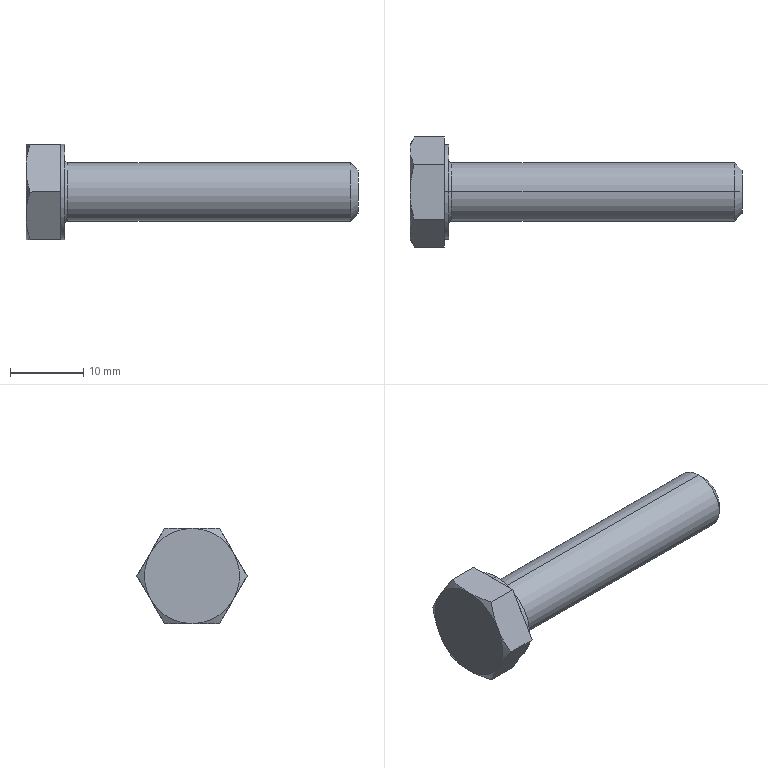Part | SolidWorks | features BaseBody 1 | 1 solid | 29 faces | box 45.3 x 15.011 x 13 mm | volume 2765 mm3 | plane 15 | cone 8 | cylinder 4 | torus 2 | commonest cylinder face diameters 8 x2 13 x2
STEP:
#1=CARTESIAN_POINT('',(5.7,0.,4.));
#2=VERTEX_POINT('',#1);
#3=CARTESIAN_POINT('',(5.3,0.,4.4));
#4=VERTEX_POINT('',#3);
#5=CARTESIAN_POINT('',(5.7,0.,4.4));
#6=DIRECTION('',(0.,1.,0.));
#7=DIRECTION('',(0.,0.,1.));
#8=AXIS2_PLACEMENT_3D('',#5,#6,#7);
#9=CIRCLE('',#8,0.4);
#10=EDGE_CURVE('',#2,#4,#9,.T.);
#11=ORIENTED_EDGE('',*,*,#10,.F.);
#12=CARTESIAN_POINT('',(5.7,0.,-4.));
#13=VERTEX_POINT('',#12);
#14=CARTESIAN_POINT('',(5.7,0.,0.));
#15=DIRECTION('',(1.,0.,0.));
#16=DIRECTION('',(0.,0.,-1.));
#17=AXIS2_PLACEMENT_3D('',#14,#15,#16);
#18=CIRCLE('',#17,4.);
#19=EDGE_CURVE('',#13,#2,#18,.T.);
#20=ORIENTED_EDGE('',*,*,#19,.F.);
#21=CARTESIAN_POINT('',(5.3,0.,-4.4));
#22=VERTEX_POINT('',#21);
#23=CARTESIAN_POINT('',(5.7,0.,-4.4));
#24=DIRECTION('',(0.,-1.,0.));
#25=DIRECTION('',(0.,0.,-1.));
#26=AXIS2_PLACEMENT_3D('',#23,#24,#25);
#27=CIRCLE('',#26,0.4);
#28=EDGE_CURVE('',#13,#22,#27,.T.);
#29=ORIENTED_EDGE('',*,*,#28,.T.);
#30=CARTESIAN_POINT('',(5.3,0.,0.));
#31=DIRECTION('',(-1.,0.,0.));
#32=DIRECTION('',(0.,0.,-1.));
#33=AXIS2_PLACEMENT_3D('',#30,#31,#32);
#34=CIRCLE('',#33,4.4);
#35=EDGE_CURVE('',#4,#22,#34,.T.);
#36=ORIENTED_EDGE('',*,*,#35,.F.);
#37=EDGE_LOOP('',(#11,#20,#29,#36));
#38=FACE_OUTER_BOUND('',#37,.T.);
#39=CARTESIAN_POINT('',(5.7,0.,0.));
#40=DIRECTION('',(1.,0.,0.));
#41=DIRECTION('',(0.,0.,-1.));
#42=AXIS2_PLACEMENT_3D('',#39,#40,#41);
#43=TOROIDAL_SURFACE('',#42,4.4,0.4);
#44=ADVANCED_FACE('',(#38),#43,.F.);
#45=CARTESIAN_POINT('',(45.3,0.,-3.));
#46=VERTEX_POINT('',#45);
#47=CARTESIAN_POINT('',(44.3,0.,-4.));
#48=VERTEX_POINT('',#47);
#49=CARTESIAN_POINT('',(44.3,0.,-4.));
#50=DIRECTION('',(-0.7071,0.,-0.7071));
#51=VECTOR('',#50,1000.);
#52=LINE('',#49,#51);
#53=EDGE_CURVE('',#46,#48,#52,.T.);
#54=ORIENTED_EDGE('',*,*,#53,.F.);
#55=CARTESIAN_POINT('',(45.3,0.,3.));
#56=VERTEX_POINT('',#55);
#57=CARTESIAN_POINT('',(45.3,0.,0.));
#58=DIRECTION('',(1.,0.,0.));
#59=DIRECTION('',(0.,0.,1.));
#60=AXIS2_PLACEMENT_3D('',#57,#58,#59);
#61=CIRCLE('',#60,3.);
#62=EDGE_CURVE('',#56,#46,#61,.T.);
#63=ORIENTED_EDGE('',*,*,#62,.F.);
#64=CARTESIAN_POINT('',(44.3,0.,4.));
#65=VERTEX_POINT('',#64);
#66=CARTESIAN_POINT('',(44.3,0.,4.));
#67=DIRECTION('',(-0.7071,0.,0.7071));
#68=VECTOR('',#67,1000.);
#69=LINE('',#66,#68);
#70=EDGE_CURVE('',#56,#65,#69,.T.);
#71=ORIENTED_EDGE('',*,*,#70,.T.);
#72=CARTESIAN_POINT('',(44.3,0.,0.));
#73=DIRECTION('',(-1.,0.,0.));
#74=DIRECTION('',(0.,0.,1.));
#75=AXIS2_PLACEMENT_3D('',#72,#73,#74);
#76=CIRCLE('',#75,4.);
#77=EDGE_CURVE('',#48,#65,#76,.T.);
#78=ORIENTED_EDGE('',*,*,#77,.F.);
#79=EDGE_LOOP('',(#54,#63,#71,#78));
#80=FACE_OUTER_BOUND('',#79,.T.);
#81=CARTESIAN_POINT('',(44.3,0.,0.));
#82=DIRECTION('',(-1.,0.,0.));
#83=DIRECTION('',(0.,0.,1.));
#84=AXIS2_PLACEMENT_3D('',#81,#82,#83);
#85=CONICAL_SURFACE('',#84,4.,0.7854);
#86=ADVANCED_FACE('',(#80),#85,.T.);
#87=CARTESIAN_POINT('',(5.3,0.,0.));
#88=DIRECTION('',(-1.,0.,0.));
#89=DIRECTION('',(0.,0.,-1.));
#90=AXIS2_PLACEMENT_3D('',#87,#88,#89);
#91=CIRCLE('',#90,4.4);
#92=EDGE_CURVE('',#22,#4,#91,.T.);
#93=ORIENTED_EDGE('',*,*,#92,.T.);
#94=ORIENTED_EDGE('',*,*,#35,.T.);
#95=EDGE_LOOP('',(#93,#94));
#96=FACE_BOUND('',#95,.T.);
#97=CARTESIAN_POINT('',(5.3,0.,6.5));
#98=VERTEX_POINT('',#97);
#99=CARTESIAN_POINT('',(5.3,0.,-6.5));
#100=VERTEX_POINT('',#99);
#101=CARTESIAN_POINT('',(5.3,0.,0.));
#102=DIRECTION('',(1.,0.,0.));
#103=DIRECTION('',(0.,0.,-1.));
#104=AXIS2_PLACEMENT_3D('',#101,#102,#103);
#105=CIRCLE('',#104,6.5);
#106=EDGE_CURVE('',#98,#100,#105,.T.);
#107=ORIENTED_EDGE('',*,*,#106,.T.);
#108=CARTESIAN_POINT('',(5.3,0.,0.));
#109=DIRECTION('',(1.,0.,0.));
#110=DIRECTION('',(0.,0.,-1.));
#111=AXIS2_PLACEMENT_3D('',#108,#109,#110);
#112=CIRCLE('',#111,6.5);
#113=EDGE_CURVE('',#100,#98,#112,.T.);
#114=ORIENTED_EDGE('',*,*,#113,.T.);
#115=EDGE_LOOP('',(#107,#114));
#116=FACE_OUTER_BOUND('',#115,.T.);
#117=CARTESIAN_POINT('',(5.3,7.506,0.));
#118=DIRECTION('',(1.,0.,0.));
#119=DIRECTION('',(0.,1.,0.));
#120=AXIS2_PLACEMENT_3D('',#117,#118,#119);
#121=PLANE('',#120);
#122=ADVANCED_FACE('',(#96,#116),#121,.T.);
#123=CARTESIAN_POINT('',(0.,0.,-4.));
#124=DIRECTION('',(-1.,0.,0.));
#125=VECTOR('',#124,1000.);
#126=LINE('',#123,#125);
#127=EDGE_CURVE('',#48,#13,#126,.T.);
#128=ORIENTED_EDGE('',*,*,#127,.F.);
#129=ORIENTED_EDGE('',*,*,#77,.T.);
#130=CARTESIAN_POINT('',(0.,0.,4.));
#131=DIRECTION('',(-1.,0.,0.));
#132=VECTOR('',#131,1000.);
#133=LINE('',#130,#132);
#134=EDGE_CURVE('',#65,#2,#133,.T.);
#135=ORIENTED_EDGE('',*,*,#134,.T.);
#136=CARTESIAN_POINT('',(5.7,0.,0.));
#137=DIRECTION('',(1.,0.,0.));
#138=DIRECTION('',(0.,0.,-1.));
#139=AXIS2_PLACEMENT_3D('',#136,#137,#138);
#140=CIRCLE('',#139,4.);
#141=EDGE_CURVE('',#2,#13,#140,.T.);
#142=ORIENTED_EDGE('',*,*,#141,.T.);
#143=EDGE_LOOP('',(#128,#129,#135,#142));
#144=FACE_OUTER_BOUND('',#143,.T.);
#145=CARTESIAN_POINT('',(0.,0.,0.));
#146=DIRECTION('',(-1.,0.,0.));
#147=DIRECTION('',(0.,0.,1.));
#148=AXIS2_PLACEMENT_3D('',#145,#146,#147);
#149=CYLINDRICAL_SURFACE('',#148,4.);
#150=ADVANCED_FACE('',(#144),#149,.T.);
#151=ORIENTED_EDGE('',*,*,#62,.T.);
#152=CARTESIAN_POINT('',(45.3,0.,0.));
#153=DIRECTION('',(1.,0.,0.));
#154=DIRECTION('',(0.,0.,1.));
#155=AXIS2_PLACEMENT_3D('',#152,#153,#154);
#156=CIRCLE('',#155,3.);
#157=EDGE_CURVE('',#46,#56,#156,.T.);
#158=ORIENTED_EDGE('',*,*,#157,.T.);
#159=EDGE_LOOP('',(#151,#158));
#160=FACE_OUTER_BOUND('',#159,.T.);
#161=CARTESIAN_POINT('',(45.3,0.,0.));
#162=DIRECTION('',(-1.,0.,0.));
#163=DIRECTION('',(0.,0.,1.));
#164=AXIS2_PLACEMENT_3D('',#161,#162,#163);
#165=PLANE('',#164);
#166=ADVANCED_FACE('',(#160),#165,.F.);
#167=CARTESIAN_POINT('',(4.7,0.,-6.5));
#168=VERTEX_POINT('',#167);
#169=CARTESIAN_POINT('',(0.,0.,-6.5));
#170=DIRECTION('',(-1.,0.,0.));
#171=VECTOR('',#170,1000.);
#172=LINE('',#169,#171);
#173=EDGE_CURVE('',#100,#168,#172,.T.);
#174=ORIENTED_EDGE('',*,*,#173,.F.);
#175=ORIENTED_EDGE('',*,*,#106,.F.);
#176=CARTESIAN_POINT('',(4.7,0.,6.5));
#177=VERTEX_POINT('',#176);
#178=CARTESIAN_POINT('',(0.,0.,6.5));
#179=DIRECTION('',(-1.,0.,0.));
#180=VECTOR('',#179,1000.);
#181=LINE('',#178,#180);
#182=EDGE_CURVE('',#98,#177,#181,.T.);
#183=ORIENTED_EDGE('',*,*,#182,.T.);
#184=CARTESIAN_POINT('',(4.7,-5.629,3.25));
#185=VERTEX_POINT('',#184);
#186=CARTESIAN_POINT('',(4.7,0.,0.));
#187=DIRECTION('',(-1.,0.,0.));
#188=DIRECTION('',(0.,0.,1.));
#189=AXIS2_PLACEMENT_3D('',#186,#187,#188);
#190=CIRCLE('',#189,6.5);
#191=EDGE_CURVE('',#185,#177,#190,.T.);
#192=ORIENTED_EDGE('',*,*,#191,.F.);
#193=CARTESIAN_POINT('',(4.7,-5.629,-3.25));
#194=VERTEX_POINT('',#193);
#195=CARTESIAN_POINT('',(4.7,0.,0.));
#196=DIRECTION('',(-1.,0.,0.));
#197=DIRECTION('',(0.,0.,1.));
#198=AXIS2_PLACEMENT_3D('',#195,#196,#197);
#199=CIRCLE('',#198,6.5);
#200=EDGE_CURVE('',#194,#185,#199,.T.);
#201=ORIENTED_EDGE('',*,*,#200,.F.);
#202=CARTESIAN_POINT('',(4.7,0.,0.));
#203=DIRECTION('',(-1.,0.,0.));
#204=DIRECTION('',(0.,0.,1.));
#205=AXIS2_PLACEMENT_3D('',#202,#203,#204);
#206=CIRCLE('',#205,6.5);
#207=EDGE_CURVE('',#168,#194,#206,.T.);
#208=ORIENTED_EDGE('',*,*,#207,.F.);
#209=EDGE_LOOP('',(#174,#175,#183,#192,#201,#208));
#210=FACE_OUTER_BOUND('',#209,.T.);
#211=CARTESIAN_POINT('',(0.,0.,0.));
#212=DIRECTION('',(-1.,0.,0.));
#213=DIRECTION('',(0.,0.,1.));
#214=AXIS2_PLACEMENT_3D('',#211,#212,#213);
#215=CYLINDRICAL_SURFACE('',#214,6.5);
#216=ADVANCED_FACE('',(#210),#215,.T.);
#217=CARTESIAN_POINT('',(4.7,-3.753,-6.5));
#218=VERTEX_POINT('',#217);
#219=CARTESIAN_POINT('',(4.7,-3.753,-6.5));
#220=DIRECTION('',(0.,0.5,-0.866));
#221=VECTOR('',#220,1000.);
#222=LINE('',#219,#221);
#223=EDGE_CURVE('',#194,#218,#222,.T.);
#224=ORIENTED_EDGE('',*,*,#223,.T.);
#225=CARTESIAN_POINT('',(4.7,3.753,-6.5));
#226=DIRECTION('',(0.,1.,0.));
#227=VECTOR('',#226,1000.);
#228=LINE('',#225,#227);
#229=EDGE_CURVE('',#218,#168,#228,.T.);
#230=ORIENTED_EDGE('',*,*,#229,.T.);
#231=ORIENTED_EDGE('',*,*,#207,.T.);
#232=EDGE_LOOP('',(#224,#230,#231));
#233=FACE_OUTER_BOUND('',#232,.T.);
#234=CARTESIAN_POINT('',(4.7,6.5,0.));
#235=DIRECTION('',(1.,0.,0.));
#236=DIRECTION('',(0.,1.,0.));
#237=AXIS2_PLACEMENT_3D('',#234,#235,#236);
#238=PLANE('',#237);
#239=ADVANCED_FACE('',(#233),#238,.T.);
#240=CARTESIAN_POINT('',(4.7,-7.506,0.));
#241=VERTEX_POINT('',#240);
#242=CARTESIAN_POINT('',(4.7,-7.506,0.));
#243=DIRECTION('',(0.,-0.5,-0.866));
#244=VECTOR('',#243,1000.);
#245=LINE('',#242,#244);
#246=EDGE_CURVE('',#185,#241,#245,.T.);
#247=ORIENTED_EDGE('',*,*,#246,.T.);
#248=CARTESIAN_POINT('',(4.7,-3.753,-6.5));
#249=DIRECTION('',(0.,0.5,-0.866));
#250=VECTOR('',#249,1000.);
#251=LINE('',#248,#250);
#252=EDGE_CURVE('',#241,#194,#251,.T.);
#253=ORIENTED_EDGE('',*,*,#252,.T.);
#254=ORIENTED_EDGE('',*,*,#200,.T.);
#255=EDGE_LOOP('',(#247,#253,#254));
#256=FACE_OUTER_BOUND('',#255,.T.);
#257=CARTESIAN_POINT('',(4.7,6.5,0.));
#258=DIRECTION('',(1.,0.,0.));
#259=DIRECTION('',(0.,1.,0.));
#260=AXIS2_PLACEMENT_3D('',#257,#258,#259);
#261=PLANE('',#260);
#262=ADVANCED_FACE('',(#256),#261,.T.);
#263=CARTESIAN_POINT('',(4.7,-3.753,6.5));
#264=VERTEX_POINT('',#263);
#265=CARTESIAN_POINT('',(4.7,3.753,6.5));
#266=DIRECTION('',(0.,-1.,0.));
#267=VECTOR('',#266,1000.);
#268=LINE('',#265,#267);
#269=EDGE_CURVE('',#177,#264,#268,.T.);
#270=ORIENTED_EDGE('',*,*,#269,.T.);
#271=CARTESIAN_POINT('',(4.7,-7.506,0.));
#272=DIRECTION('',(0.,-0.5,-0.866));
#273=VECTOR('',#272,1000.);
#274=LINE('',#271,#273);
#275=EDGE_CURVE('',#264,#185,#274,.T.);
#276=ORIENTED_EDGE('',*,*,#275,.T.);
#277=ORIENTED_EDGE('',*,*,#191,.T.);
#278=EDGE_LOOP('',(#270,#276,#277));
#279=FACE_OUTER_BOUND('',#278,.T.);
#280=CARTESIAN_POINT('',(4.7,6.5,0.));
#281=DIRECTION('',(1.,0.,0.));
#282=DIRECTION('',(0.,1.,0.));
#283=AXIS2_PLACEMENT_3D('',#280,#281,#282);
#284=PLANE('',#283);
#285=ADVANCED_FACE('',(#279),#284,.T.);
#286=CARTESIAN_POINT('',(4.7,5.629,3.25));
#287=VERTEX_POINT('',#286);
#288=CARTESIAN_POINT('',(4.7,3.753,6.5));
#289=VERTEX_POINT('',#288);
#290=CARTESIAN_POINT('',(4.7,7.506,0.));
#291=DIRECTION('',(0.,-0.5,0.866));
#292=VECTOR('',#291,1000.);
#293=LINE('',#290,#292);
#294=EDGE_CURVE('',#287,#289,#293,.T.);
#295=ORIENTED_EDGE('',*,*,#294,.T.);
#296=CARTESIAN_POINT('',(4.7,3.753,6.5));
#297=DIRECTION('',(0.,-1.,0.));
#298=VECTOR('',#297,1000.);
#299=LINE('',#296,#298);
#300=EDGE_CURVE('',#289,#177,#299,.T.);
#301=ORIENTED_EDGE('',*,*,#300,.T.);
#302=CARTESIAN_POINT('',(4.7,0.,0.));
#303=DIRECTION('',(-1.,0.,0.));
#304=DIRECTION('',(0.,0.,1.));
#305=AXIS2_PLACEMENT_3D('',#302,#303,#304);
#306=CIRCLE('',#305,6.5);
#307=EDGE_CURVE('',#177,#287,#306,.T.);
#308=ORIENTED_EDGE('',*,*,#307,.T.);
#309=EDGE_LOOP('',(#295,#301,#308));
#310=FACE_OUTER_BOUND('',#309,.T.);
#311=CARTESIAN_POINT('',(4.7,6.5,0.));
#312=DIRECTION('',(1.,0.,0.));
#313=DIRECTION('',(0.,1.,0.));
#314=AXIS2_PLACEMENT_3D('',#311,#312,#313);
#315=PLANE('',#314);
#316=ADVANCED_FACE('',(#310),#315,.T.);
#317=CARTESIAN_POINT('',(4.7,5.629,-3.25));
#318=VERTEX_POINT('',#317);
#319=CARTESIAN_POINT('',(4.7,7.506,0.));
#320=VERTEX_POINT('',#319);
#321=CARTESIAN_POINT('',(4.7,3.753,-6.5));
#322=DIRECTION('',(0.,0.5,0.866));
#323=VECTOR('',#322,1000.);
#324=LINE('',#321,#323);
#325=EDGE_CURVE('',#318,#320,#324,.T.);
#326=ORIENTED_EDGE('',*,*,#325,.T.);
#327=CARTESIAN_POINT('',(4.7,7.506,0.));
#328=DIRECTION('',(0.,-0.5,0.866));
#329=VECTOR('',#328,1000.);
#330=LINE('',#327,#329);
#331=EDGE_CURVE('',#320,#287,#330,.T.);
#332=ORIENTED_EDGE('',*,*,#331,.T.);
#333=CARTESIAN_POINT('',(4.7,0.,0.));
#334=DIRECTION('',(-1.,0.,0.));
#335=DIRECTION('',(0.,0.,1.));
#336=AXIS2_PLACEMENT_3D('',#333,#334,#335);
#337=CIRCLE('',#336,6.5);
#338=EDGE_CURVE('',#287,#318,#337,.T.);
#339=ORIENTED_EDGE('',*,*,#338,.T.);
#340=EDGE_LOOP('',(#326,#332,#339));
#341=FACE_OUTER_BOUND('',#340,.T.);
#342=CARTESIAN_POINT('',(4.7,6.5,0.));
#343=DIRECTION('',(1.,0.,0.));
#344=DIRECTION('',(0.,1.,0.));
#345=AXIS2_PLACEMENT_3D('',#342,#343,#344);
#346=PLANE('',#345);
#347=ADVANCED_FACE('',(#341),#346,.T.);
#348=CARTESIAN_POINT('',(4.7,3.753,-6.5));
#349=VERTEX_POINT('',#348);
#350=CARTESIAN_POINT('',(4.7,3.753,-6.5));
#351=DIRECTION('',(0.,0.5,0.866));
#352=VECTOR('',#351,1000.);
#353=LINE('',#350,#352);
#354=EDGE_CURVE('',#349,#318,#353,.T.);
#355=ORIENTED_EDGE('',*,*,#354,.T.);
#356=CARTESIAN_POINT('',(4.7,0.,0.));
#357=DIRECTION('',(-1.,0.,0.));
#358=DIRECTION('',(0.,0.,1.));
#359=AXIS2_PLACEMENT_3D('',#356,#357,#358);
#360=CIRCLE('',#359,6.5);
#361=EDGE_CURVE('',#318,#168,#360,.T.);
#362=ORIENTED_EDGE('',*,*,#361,.T.);
#363=CARTESIAN_POINT('',(4.7,3.753,-6.5));
#364=DIRECTION('',(0.,1.,0.));
#365=VECTOR('',#364,1000.);
#366=LINE('',#363,#365);
#367=EDGE_CURVE('',#168,#349,#366,.T.);
#368=ORIENTED_EDGE('',*,*,#367,.T.);
#369=EDGE_LOOP('',(#355,#362,#368));
#370=FACE_OUTER_BOUND('',#369,.T.);
#371=CARTESIAN_POINT('',(4.7,6.5,0.));
#372=DIRECTION('',(1.,0.,0.));
#373=DIRECTION('',(0.,1.,0.));
#374=AXIS2_PLACEMENT_3D('',#371,#372,#373);
#375=PLANE('',#374);
#376=ADVANCED_FACE('',(#370),#375,.T.);
#377=CARTESIAN_POINT('',(0.,0.,-6.5));
#378=VERTEX_POINT('',#377);
#379=CARTESIAN_POINT('',(0.,5.629,-3.25));
#380=VERTEX_POINT('',#379);
#381=CARTESIAN_POINT('',(0.,0.,0.));
#382=DIRECTION('',(1.,0.,0.));
#383=DIRECTION('',(0.,0.,-1.));
#384=AXIS2_PLACEMENT_3D('',#381,#382,#383);
#385=CIRCLE('',#384,6.5);
#386=EDGE_CURVE('',#378,#380,#385,.T.);
#387=ORIENTED_EDGE('',*,*,#386,.F.);
#388=CARTESIAN_POINT('',(0.,-5.629,-3.25));
#389=VERTEX_POINT('',#388);
#390=CARTESIAN_POINT('',(0.,0.,0.));
#391=DIRECTION('',(1.,0.,0.));
#392=DIRECTION('',(0.,0.,-1.));
#393=AXIS2_PLACEMENT_3D('',#390,#391,#392);
#394=CIRCLE('',#393,6.5);
#395=EDGE_CURVE('',#389,#378,#394,.T.);
#396=ORIENTED_EDGE('',*,*,#395,.F.);
#397=CARTESIAN_POINT('',(0.,-5.629,3.25));
#398=VERTEX_POINT('',#397);
#399=CARTESIAN_POINT('',(0.,0.,0.));
#400=DIRECTION('',(1.,0.,0.));
#401=DIRECTION('',(0.,0.,-1.));
#402=AXIS2_PLACEMENT_3D('',#399,#400,#401);
#403=CIRCLE('',#402,6.5);
#404=EDGE_CURVE('',#398,#389,#403,.T.);
#405=ORIENTED_EDGE('',*,*,#404,.F.);
#406=CARTESIAN_POINT('',(0.,0.,6.5));
#407=VERTEX_POINT('',#406);
#408=CARTESIAN_POINT('',(0.,0.,0.));
#409=DIRECTION('',(1.,0.,0.));
#410=DIRECTION('',(0.,0.,-1.));
#411=AXIS2_PLACEMENT_3D('',#408,#409,#410);
#412=CIRCLE('',#411,6.5);
#413=EDGE_CURVE('',#407,#398,#412,.T.);
#414=ORIENTED_EDGE('',*,*,#413,.F.);
#415=CARTESIAN_POINT('',(0.,5.629,3.25));
#416=VERTEX_POINT('',#415);
#417=CARTESIAN_POINT('',(0.,0.,0.));
#418=DIRECTION('',(-1.,0.,0.));
#419=DIRECTION('',(0.,0.,1.));
#420=AXIS2_PLACEMENT_3D('',#417,#418,#419);
#421=CIRCLE('',#420,6.5);
#422=EDGE_CURVE('',#407,#416,#421,.T.);
#423=ORIENTED_EDGE('',*,*,#422,.T.);
#424=CARTESIAN_POINT('',(0.,0.,0.));
#425=DIRECTION('',(1.,0.,0.));
#426=DIRECTION('',(0.,0.,-1.));
#427=AXIS2_PLACEMENT_3D('',#424,#425,#426);
#428=CIRCLE('',#427,6.5);
#429=EDGE_CURVE('',#380,#416,#428,.T.);
#430=ORIENTED_EDGE('',*,*,#429,.F.);
#431=EDGE_LOOP('',(#387,#396,#405,#414,#423,#430));
#432=FACE_OUTER_BOUND('',#431,.T.);
#433=CARTESIAN_POINT('',(0.,7.506,0.));
#434=DIRECTION('',(1.,0.,0.));
#435=DIRECTION('',(0.,1.,0.));
#436=AXIS2_PLACEMENT_3D('',#433,#434,#435);
#437=PLANE('',#436);
#438=ADVANCED_FACE('',(#432),#437,.F.);
#439=CARTESIAN_POINT('',(0.5806,3.753,-6.5));
#440=VERTEX_POINT('',#439);
#441=CARTESIAN_POINT('',(0.,5.629,-3.25));
#442=CARTESIAN_POINT('',(0.,5.549,-3.388));
#443=CARTESIAN_POINT('',(0.003356,5.47,-3.525));
#444=CARTESIAN_POINT('',(0.01342,5.351,-3.732));
#445=CARTESIAN_POINT('',(0.01762,5.311,-3.801));
#446=CARTESIAN_POINT('',(0.02769,5.232,-3.939));
#447=CARTESIAN_POINT('',(0.0337,5.191,-4.009));
#448=CARTESIAN_POINT('',(0.05342,5.073,-4.213));
#449=CARTESIAN_POINT('',(0.0697,4.995,-4.348));
#450=CARTESIAN_POINT('',(0.09881,4.877,-4.552));
#451=CARTESIAN_POINT('',(0.1145,4.818,-4.654));
#452=CARTESIAN_POINT('',(0.132,4.759,-4.757));
#453=CARTESIAN_POINT('',(0.1441,4.72,-4.825));
#454=CARTESIAN_POINT('',(0.1506,4.699,-4.861));
#455=CARTESIAN_POINT('',(0.2548,4.377,-5.419));
#456=CARTESIAN_POINT('',(0.3961,4.072,-5.947));
#457=CARTESIAN_POINT('',(0.5806,3.753,-6.5));
#458=B_SPLINE_CURVE_WITH_KNOTS('',3,(#441,#442,#443,#444,#445,#446,#447,#448,#449,#450,#451,#452,#453,#454,#455,#456,#457),.UNSPECIFIED.,.F.,.F.,(4,2,2,2,2,1,2,2,4),(0.,0.125,0.1875,0.25,0.375,0.4375,0.4687,0.5,1.),.UNSPECIFIED.);
#459=EDGE_CURVE('',#380,#440,#458,.T.);
#460=ORIENTED_EDGE('',*,*,#459,.T.);
#461=CARTESIAN_POINT('',(0.5806,3.753,-6.5));
#462=CARTESIAN_POINT('',(0.4887,3.435,-6.5));
#463=CARTESIAN_POINT('',(0.4075,3.123,-6.5));
#464=CARTESIAN_POINT('',(0.3018,2.663,-6.5));
#465=CARTESIAN_POINT('',(0.2693,2.511,-6.5));
#466=CARTESIAN_POINT('',(0.2245,2.283,-6.5));
#467=CARTESIAN_POINT('',(0.2031,2.169,-6.5));
#468=CARTESIAN_POINT('',(0.1832,2.056,-6.5));
#469=CARTESIAN_POINT('',(0.1703,1.98,-6.5));
#470=CARTESIAN_POINT('',(0.1643,1.945,-6.5));
#471=CARTESIAN_POINT('',(0.132,1.746,-6.5));
#472=CARTESIAN_POINT('',(0.1093,1.587,-6.5));
#473=CARTESIAN_POINT('',(0.07994,1.351,-6.5));
#474=CARTESIAN_POINT('',(0.07094,1.272,-6.5));
#475=CARTESIAN_POINT('',(0.05452,1.114,-6.5));
#476=CARTESIAN_POINT('',(0.0472,1.036,-6.5));
#477=CARTESIAN_POINT('',(0.01349,0.6346,-6.5));
#478=CARTESIAN_POINT('',(0.,0.3183,-6.5));
#479=CARTESIAN_POINT('',(0.,0.,-6.5));
#480=B_SPLINE_CURVE_WITH_KNOTS('',3,(#461,#462,#463,#464,#465,#466,#467,#468,#469,#470,#471,#472,#473,#474,#475,#476,#477,#478,#479),.UNSPECIFIED.,.F.,.F.,(4,2,2,1,2,2,2,2,2,4),(0.,0.25,0.375,0.4375,0.4688,0.5,0.625,0.6875,0.75,1.),.UNSPECIFIED.);
#481=EDGE_CURVE('',#440,#378,#480,.T.);
#482=ORIENTED_EDGE('',*,*,#481,.T.);
#483=ORIENTED_EDGE('',*,*,#386,.T.);
#484=EDGE_LOOP('',(#460,#482,#483));
#485=FACE_OUTER_BOUND('',#484,.T.);
#486=CARTESIAN_POINT('',(0.,0.,0.));
#487=DIRECTION('',(1.,0.,0.));
#488=DIRECTION('',(0.,0.,-1.));
#489=AXIS2_PLACEMENT_3D('',#486,#487,#488);
#490=CONICAL_SURFACE('',#489,6.5,1.047);
#491=ADVANCED_FACE('',(#485),#490,.T.);
#492=CARTESIAN_POINT('',(0.5806,7.506,0.));
#493=VERTEX_POINT('',#492);
#494=CARTESIAN_POINT('',(0.,5.629,3.25));
#495=CARTESIAN_POINT('',(0.,5.709,3.112));
#496=CARTESIAN_POINT('',(0.003356,5.788,2.974));
#497=CARTESIAN_POINT('',(0.01342,5.907,2.768));
#498=CARTESIAN_POINT('',(0.01762,5.947,2.699));
#499=CARTESIAN_POINT('',(0.02769,6.027,2.561));
#500=CARTESIAN_POINT('',(0.0337,6.067,2.491));
#501=CARTESIAN_POINT('',(0.05342,6.185,2.287));
#502=CARTESIAN_POINT('',(0.0697,6.263,2.152));
#503=CARTESIAN_POINT('',(0.09881,6.381,1.948));
#504=CARTESIAN_POINT('',(0.1145,6.44,1.846));
#505=CARTESIAN_POINT('',(0.132,6.499,1.743));
#506=CARTESIAN_POINT('',(0.1441,6.539,1.675));
#507=CARTESIAN_POINT('',(0.1506,6.559,1.639));
#508=CARTESIAN_POINT('',(0.2548,6.881,1.081));
#509=CARTESIAN_POINT('',(0.3961,7.186,0.5534));
#510=CARTESIAN_POINT('',(0.5806,7.506,0.));
#511=B_SPLINE_CURVE_WITH_KNOTS('',3,(#494,#495,#496,#497,#498,#499,#500,#501,#502,#503,#504,#505,#506,#507,#508,#509,#510),.UNSPECIFIED.,.F.,.F.,(4,2,2,2,2,1,2,2,4),(0.,0.125,0.1875,0.25,0.375,0.4375,0.4687,0.5,1.),.UNSPECIFIED.);
#512=EDGE_CURVE('',#416,#493,#511,.T.);
#513=ORIENTED_EDGE('',*,*,#512,.T.);
#514=CARTESIAN_POINT('',(0.5806,7.506,0.));
#515=CARTESIAN_POINT('',(0.4882,7.346,-0.277));
#516=CARTESIAN_POINT('',(0.4067,7.189,-0.5478));
#517=CARTESIAN_POINT('',(0.3006,6.958,-0.9485));
#518=CARTESIAN_POINT('',(0.268,6.881,-1.081));
#519=CARTESIAN_POINT('',(0.2231,6.767,-1.279));
#520=CARTESIAN_POINT('',(0.2016,6.71,-1.378));
#521=CARTESIAN_POINT('',(0.1817,6.653,-1.477));
#522=CARTESIAN_POINT('',(0.1688,6.615,-1.543));
#523=CARTESIAN_POINT('',(0.1627,6.597,-1.574));
#524=CARTESIAN_POINT('',(0.1307,6.498,-1.745));
#525=CARTESIAN_POINT('',(0.1083,6.419,-1.882));
#526=CARTESIAN_POINT('',(0.07923,6.302,-2.085));
#527=CARTESIAN_POINT('',(0.07033,6.262,-2.153));
#528=CARTESIAN_POINT('',(0.05409,6.184,-2.289));
#529=CARTESIAN_POINT('',(0.04688,6.146,-2.355));
#530=CARTESIAN_POINT('',(0.01339,5.946,-2.701));
#531=CARTESIAN_POINT('',(0.,5.788,-2.975));
#532=CARTESIAN_POINT('',(0.,5.629,-3.25));
#533=B_SPLINE_CURVE_WITH_KNOTS('',3,(#514,#515,#516,#517,#518,#519,#520,#521,#522,#523,#524,#525,#526,#527,#528,#529,#530,#531,#532),.UNSPECIFIED.,.F.,.F.,(4,2,2,1,2,2,2,2,2,4),(0.,0.25,0.375,0.4375,0.4687,0.5,0.625,0.6875,0.75,1.),.UNSPECIFIED.);
#534=EDGE_CURVE('',#493,#380,#533,.T.);
#535=ORIENTED_EDGE('',*,*,#534,.T.);
#536=ORIENTED_EDGE('',*,*,#429,.T.);
#537=EDGE_LOOP('',(#513,#535,#536));
#538=FACE_OUTER_BOUND('',#537,.T.);
#539=CARTESIAN_POINT('',(0.,0.,0.));
#540=DIRECTION('',(1.,0.,0.));
#541=DIRECTION('',(0.,0.,-1.));
#542=AXIS2_PLACEMENT_3D('',#539,#540,#541);
#543=CONICAL_SURFACE('',#542,6.5,1.047);
#544=ADVANCED_FACE('',(#538),#543,.T.);
#545=CARTESIAN_POINT('',(0.5806,3.753,6.5));
#546=VERTEX_POINT('',#545);
#547=CARTESIAN_POINT('',(0.,0.,6.5));
#548=CARTESIAN_POINT('',(0.,0.1591,6.5));
#549=CARTESIAN_POINT('',(0.003371,0.3178,6.5));
#550=CARTESIAN_POINT('',(0.01349,0.5563,6.5));
#551=CARTESIAN_POINT('',(0.0177,0.6359,6.5));
#552=CARTESIAN_POINT('',(0.02781,0.7955,6.5));
#553=CARTESIAN_POINT('',(0.03382,0.8767,6.5));
#554=CARTESIAN_POINT('',(0.05373,1.114,6.5));
#555=CARTESIAN_POINT('',(0.07015,1.272,6.5));
#556=CARTESIAN_POINT('',(0.09949,1.508,6.5));
#557=CARTESIAN_POINT('',(0.1153,1.627,6.5));
#558=CARTESIAN_POINT('',(0.133,1.746,6.5));
#559=CARTESIAN_POINT('',(0.1451,1.825,6.5));
#560=CARTESIAN_POINT('',(0.1517,1.867,6.5));
#561=CARTESIAN_POINT('',(0.2559,2.509,6.5));
#562=CARTESIAN_POINT('',(0.3968,3.116,6.5));
#563=CARTESIAN_POINT('',(0.5806,3.753,6.5));
#564=B_SPLINE_CURVE_WITH_KNOTS('',3,(#547,#548,#549,#550,#551,#552,#553,#554,#555,#556,#557,#558,#559,#560,#561,#562,#563),.UNSPECIFIED.,.F.,.F.,(4,2,2,2,2,1,2,2,4),(0.,0.125,0.1875,0.25,0.375,0.4375,0.4688,0.5,1.),.UNSPECIFIED.);
#565=EDGE_CURVE('',#407,#546,#564,.T.);
#566=ORIENTED_EDGE('',*,*,#565,.T.);
#567=CARTESIAN_POINT('',(0.5806,3.753,6.5));
#568=CARTESIAN_POINT('',(0.4882,3.913,6.223));
#569=CARTESIAN_POINT('',(0.4067,4.069,5.952));
#570=CARTESIAN_POINT('',(0.3006,4.3,5.551));
#571=CARTESIAN_POINT('',(0.268,4.377,5.419));
#572=CARTESIAN_POINT('',(0.2231,4.491,5.221));
#573=CARTESIAN_POINT('',(0.2016,4.548,5.122));
#574=CARTESIAN_POINT('',(0.1817,4.605,5.023));
#575=CARTESIAN_POINT('',(0.1688,4.643,4.957));
#576=CARTESIAN_POINT('',(0.1627,4.662,4.926));
#577=CARTESIAN_POINT('',(0.1307,4.76,4.755));
#578=CARTESIAN_POINT('',(0.1083,4.839,4.618));
#579=CARTESIAN_POINT('',(0.07923,4.957,4.415));
#580=CARTESIAN_POINT('',(0.07033,4.996,4.347));
#581=CARTESIAN_POINT('',(0.05409,5.074,4.211));
#582=CARTESIAN_POINT('',(0.04688,5.113,4.145));
#583=CARTESIAN_POINT('',(0.01339,5.312,3.799));
#584=CARTESIAN_POINT('',(0.,5.47,3.525));
#585=CARTESIAN_POINT('',(0.,5.629,3.25));
#586=B_SPLINE_CURVE_WITH_KNOTS('',3,(#567,#568,#569,#570,#571,#572,#573,#574,#575,#576,#577,#578,#579,#580,#581,#582,#583,#584,#585),.UNSPECIFIED.,.F.,.F.,(4,2,2,1,2,2,2,2,2,4),(0.,0.25,0.375,0.4375,0.4687,0.5,0.625,0.6875,0.75,1.),.UNSPECIFIED.);
#587=EDGE_CURVE('',#546,#416,#586,.T.);
#588=ORIENTED_EDGE('',*,*,#587,.T.);
#589=ORIENTED_EDGE('',*,*,#422,.F.);
#590=EDGE_LOOP('',(#566,#588,#589));
#591=FACE_OUTER_BOUND('',#590,.T.);
#592=CARTESIAN_POINT('',(0.,0.,0.));
#593=DIRECTION('',(1.,0.,0.));
#594=DIRECTION('',(0.,0.,-1.));
#595=AXIS2_PLACEMENT_3D('',#592,#593,#594);
#596=CONICAL_SURFACE('',#595,6.5,1.047);
#597=ADVANCED_FACE('',(#591),#596,.T.);
#598=CARTESIAN_POINT('',(0.5806,-3.753,6.5));
#599=VERTEX_POINT('',#598);
#600=CARTESIAN_POINT('',(0.5806,-3.753,6.5));
#601=CARTESIAN_POINT('',(0.488,-3.432,6.5));
#602=CARTESIAN_POINT('',(0.4063,-3.118,6.5));
#603=CARTESIAN_POINT('',(0.3,-2.655,6.5));
#604=CARTESIAN_POINT('',(0.2673,-2.501,6.5));
#605=CARTESIAN_POINT('',(0.2223,-2.272,6.5));
#606=CARTESIAN_POINT('',(0.2009,-2.157,6.5));
#607=CARTESIAN_POINT('',(0.1809,-2.043,6.5));
#608=CARTESIAN_POINT('',(0.168,-1.967,6.5));
#609=CARTESIAN_POINT('',(0.1619,-1.93,6.5));
#610=CARTESIAN_POINT('',(0.13,-1.733,6.5));
#611=CARTESIAN_POINT('',(0.1076,-1.575,6.5));
#612=CARTESIAN_POINT('',(0.07869,-1.34,6.5));
#613=CARTESIAN_POINT('',(0.06982,-1.262,6.5));
#614=CARTESIAN_POINT('',(0.05364,-1.105,6.5));
#615=CARTESIAN_POINT('',(0.04643,-1.028,6.5));
#616=CARTESIAN_POINT('',(0.01327,-0.6305,6.5));
#617=CARTESIAN_POINT('',(0.,-0.3164,6.5));
#618=CARTESIAN_POINT('',(0.,0.,6.5));
#619=B_SPLINE_CURVE_WITH_KNOTS('',3,(#600,#601,#602,#603,#604,#605,#606,#607,#608,#609,#610,#611,#612,#613,#614,#615,#616,#617,#618),.UNSPECIFIED.,.F.,.F.,(4,2,2,1,2,2,2,2,2,4),(0.,0.25,0.375,0.4375,0.4688,0.5,0.625,0.6875,0.75,1.),.UNSPECIFIED.);
#620=EDGE_CURVE('',#599,#407,#619,.T.);
#621=ORIENTED_EDGE('',*,*,#620,.T.);
#622=ORIENTED_EDGE('',*,*,#413,.T.);
#623=CARTESIAN_POINT('',(0.,-5.629,3.25));
#624=CARTESIAN_POINT('',(0.,-5.549,3.388));
#625=CARTESIAN_POINT('',(0.003356,-5.47,3.525));
#626=CARTESIAN_POINT('',(0.01342,-5.351,3.732));
#627=CARTESIAN_POINT('',(0.01762,-5.311,3.801));
#628=CARTESIAN_POINT('',(0.02769,-5.232,3.939));
#629=CARTESIAN_POINT('',(0.0337,-5.191,4.009));
#630=CARTESIAN_POINT('',(0.05342,-5.073,4.213));
#631=CARTESIAN_POINT('',(0.0697,-4.995,4.348));
#632=CARTESIAN_POINT('',(0.09881,-4.877,4.552));
#633=CARTESIAN_POINT('',(0.1145,-4.818,4.654));
#634=CARTESIAN_POINT('',(0.132,-4.759,4.757));
#635=CARTESIAN_POINT('',(0.1441,-4.72,4.825));
#636=CARTESIAN_POINT('',(0.1506,-4.699,4.861));
#637=CARTESIAN_POINT('',(0.2548,-4.377,5.419));
#638=CARTESIAN_POINT('',(0.3961,-4.072,5.947));
#639=CARTESIAN_POINT('',(0.5806,-3.753,6.5));
#640=B_SPLINE_CURVE_WITH_KNOTS('',3,(#623,#624,#625,#626,#627,#628,#629,#630,#631,#632,#633,#634,#635,#636,#637,#638,#639),.UNSPECIFIED.,.F.,.F.,(4,2,2,2,2,1,2,2,4),(0.,0.125,0.1875,0.25,0.375,0.4375,0.4688,0.5,1.),.UNSPECIFIED.);
#641=EDGE_CURVE('',#398,#599,#640,.T.);
#642=ORIENTED_EDGE('',*,*,#641,.T.);
#643=EDGE_LOOP('',(#621,#622,#642));
#644=FACE_OUTER_BOUND('',#643,.T.);
#645=CARTESIAN_POINT('',(0.,0.,0.));
#646=DIRECTION('',(1.,0.,0.));
#647=DIRECTION('',(0.,0.,-1.));
#648=AXIS2_PLACEMENT_3D('',#645,#646,#647);
#649=CONICAL_SURFACE('',#648,6.5,1.047);
#650=ADVANCED_FACE('',(#644),#649,.T.);
#651=CARTESIAN_POINT('',(0.5806,-7.506,0.));
#652=VERTEX_POINT('',#651);
#653=CARTESIAN_POINT('',(0.5806,-7.506,0.));
#654=CARTESIAN_POINT('',(0.4882,-7.346,0.277));
#655=CARTESIAN_POINT('',(0.4067,-7.189,0.5478));
#656=CARTESIAN_POINT('',(0.3006,-6.958,0.9485));
#657=CARTESIAN_POINT('',(0.268,-6.881,1.081));
#658=CARTESIAN_POINT('',(0.2231,-6.767,1.279));
#659=CARTESIAN_POINT('',(0.2016,-6.71,1.378));
#660=CARTESIAN_POINT('',(0.1817,-6.653,1.477));
#661=CARTESIAN_POINT('',(0.1688,-6.615,1.543));
#662=CARTESIAN_POINT('',(0.1627,-6.597,1.574));
#663=CARTESIAN_POINT('',(0.1307,-6.498,1.745));
#664=CARTESIAN_POINT('',(0.1083,-6.419,1.882));
#665=CARTESIAN_POINT('',(0.07923,-6.302,2.085));
#666=CARTESIAN_POINT('',(0.07033,-6.262,2.153));
#667=CARTESIAN_POINT('',(0.05409,-6.184,2.289));
#668=CARTESIAN_POINT('',(0.04688,-6.146,2.355));
#669=CARTESIAN_POINT('',(0.01339,-5.946,2.701));
#670=CARTESIAN_POINT('',(0.,-5.788,2.975));
#671=CARTESIAN_POINT('',(0.,-5.629,3.25));
#672=B_SPLINE_CURVE_WITH_KNOTS('',3,(#653,#654,#655,#656,#657,#658,#659,#660,#661,#662,#663,#664,#665,#666,#667,#668,#669,#670,#671),.UNSPECIFIED.,.F.,.F.,(4,2,2,1,2,2,2,2,2,4),(0.,0.25,0.375,0.4375,0.4687,0.5,0.625,0.6875,0.75,1.),.UNSPECIFIED.);
#673=EDGE_CURVE('',#652,#398,#672,.T.);
#674=ORIENTED_EDGE('',*,*,#673,.T.);
#675=ORIENTED_EDGE('',*,*,#404,.T.);
#676=CARTESIAN_POINT('',(0.,-5.629,-3.25));
#677=CARTESIAN_POINT('',(0.,-5.709,-3.112));
#678=CARTESIAN_POINT('',(0.003356,-5.788,-2.974));
#679=CARTESIAN_POINT('',(0.01342,-5.907,-2.768));
#680=CARTESIAN_POINT('',(0.01762,-5.947,-2.699));
#681=CARTESIAN_POINT('',(0.02769,-6.027,-2.561));
#682=CARTESIAN_POINT('',(0.0337,-6.067,-2.491));
#683=CARTESIAN_POINT('',(0.05342,-6.185,-2.287));
#684=CARTESIAN_POINT('',(0.0697,-6.263,-2.152));
#685=CARTESIAN_POINT('',(0.09881,-6.381,-1.948));
#686=CARTESIAN_POINT('',(0.1145,-6.44,-1.846));
#687=CARTESIAN_POINT('',(0.132,-6.499,-1.743));
#688=CARTESIAN_POINT('',(0.1441,-6.539,-1.675));
#689=CARTESIAN_POINT('',(0.1506,-6.559,-1.639));
#690=CARTESIAN_POINT('',(0.2548,-6.881,-1.081));
#691=CARTESIAN_POINT('',(0.3961,-7.186,-0.5534));
#692=CARTESIAN_POINT('',(0.5806,-7.506,0.));
#693=B_SPLINE_CURVE_WITH_KNOTS('',3,(#676,#677,#678,#679,#680,#681,#682,#683,#684,#685,#686,#687,#688,#689,#690,#691,#692),.UNSPECIFIED.,.F.,.F.,(4,2,2,2,2,1,2,2,4),(0.,0.125,0.1875,0.25,0.375,0.4375,0.4688,0.5,1.),.UNSPECIFIED.);
#694=EDGE_CURVE('',#389,#652,#693,.T.);
#695=ORIENTED_EDGE('',*,*,#694,.T.);
#696=EDGE_LOOP('',(#674,#675,#695));
#697=FACE_OUTER_BOUND('',#696,.T.);
#698=CARTESIAN_POINT('',(0.,0.,0.));
#699=DIRECTION('',(1.,0.,0.));
#700=DIRECTION('',(0.,0.,-1.));
#701=AXIS2_PLACEMENT_3D('',#698,#699,#700);
#702=CONICAL_SURFACE('',#701,6.5,1.047);
#703=ADVANCED_FACE('',(#697),#702,.T.);
#704=CARTESIAN_POINT('',(0.5806,-3.753,-6.5));
#705=VERTEX_POINT('',#704);
#706=CARTESIAN_POINT('',(0.5806,-3.753,-6.5));
#707=CARTESIAN_POINT('',(0.4882,-3.913,-6.223));
#708=CARTESIAN_POINT('',(0.4067,-4.069,-5.952));
#709=CARTESIAN_POINT('',(0.3006,-4.3,-5.551));
#710=CARTESIAN_POINT('',(0.268,-4.377,-5.419));
#711=CARTESIAN_POINT('',(0.2231,-4.491,-5.221));
#712=CARTESIAN_POINT('',(0.2016,-4.548,-5.122));
#713=CARTESIAN_POINT('',(0.1817,-4.605,-5.023));
#714=CARTESIAN_POINT('',(0.1688,-4.643,-4.957));
#715=CARTESIAN_POINT('',(0.1627,-4.662,-4.926));
#716=CARTESIAN_POINT('',(0.1307,-4.76,-4.755));
#717=CARTESIAN_POINT('',(0.1083,-4.839,-4.618));
#718=CARTESIAN_POINT('',(0.07923,-4.957,-4.415));
#719=CARTESIAN_POINT('',(0.07033,-4.996,-4.347));
#720=CARTESIAN_POINT('',(0.05409,-5.074,-4.211));
#721=CARTESIAN_POINT('',(0.04688,-5.113,-4.145));
#722=CARTESIAN_POINT('',(0.01339,-5.312,-3.799));
#723=CARTESIAN_POINT('',(0.,-5.47,-3.525));
#724=CARTESIAN_POINT('',(0.,-5.629,-3.25));
#725=B_SPLINE_CURVE_WITH_KNOTS('',3,(#706,#707,#708,#709,#710,#711,#712,#713,#714,#715,#716,#717,#718,#719,#720,#721,#722,#723,#724),.UNSPECIFIED.,.F.,.F.,(4,2,2,1,2,2,2,2,2,4),(0.,0.25,0.375,0.4375,0.4688,0.5,0.625,0.6875,0.75,1.),.UNSPECIFIED.);
#726=EDGE_CURVE('',#705,#389,#725,.T.);
#727=ORIENTED_EDGE('',*,*,#726,.T.);
#728=ORIENTED_EDGE('',*,*,#395,.T.);
#729=CARTESIAN_POINT('',(0.,0.,-6.5));
#730=CARTESIAN_POINT('',(0.,-0.1582,-6.5));
#731=CARTESIAN_POINT('',(0.003316,-0.3158,-6.5));
#732=CARTESIAN_POINT('',(0.01327,-0.5526,-6.5));
#733=CARTESIAN_POINT('',(0.01741,-0.6315,-6.5));
#734=CARTESIAN_POINT('',(0.02736,-0.7898,-6.5));
#735=CARTESIAN_POINT('',(0.03326,-0.8703,-6.5));
#736=CARTESIAN_POINT('',(0.05286,-1.105,-6.5));
#737=CARTESIAN_POINT('',(0.06904,-1.262,-6.5));
#738=CARTESIAN_POINT('',(0.09798,-1.497,-6.5));
#739=CARTESIAN_POINT('',(0.1136,-1.615,-6.5));
#740=CARTESIAN_POINT('',(0.131,-1.733,-6.5));
#741=CARTESIAN_POINT('',(0.143,-1.812,-6.5));
#742=CARTESIAN_POINT('',(0.1494,-1.853,-6.5));
#743=CARTESIAN_POINT('',(0.2537,-2.499,-6.5));
#744=CARTESIAN_POINT('',(0.3954,-3.111,-6.5));
#745=CARTESIAN_POINT('',(0.5806,-3.753,-6.5));
#746=B_SPLINE_CURVE_WITH_KNOTS('',3,(#729,#730,#731,#732,#733,#734,#735,#736,#737,#738,#739,#740,#741,#742,#743,#744,#745),.UNSPECIFIED.,.F.,.F.,(4,2,2,2,2,1,2,2,4),(0.,0.125,0.1875,0.25,0.375,0.4375,0.4688,0.5,1.),.UNSPECIFIED.);
#747=EDGE_CURVE('',#378,#705,#746,.T.);
#748=ORIENTED_EDGE('',*,*,#747,.T.);
#749=EDGE_LOOP('',(#727,#728,#748));
#750=FACE_OUTER_BOUND('',#749,.T.);
#751=CARTESIAN_POINT('',(0.,0.,0.));
#752=DIRECTION('',(1.,0.,0.));
#753=DIRECTION('',(0.,0.,-1.));
#754=AXIS2_PLACEMENT_3D('',#751,#752,#753);
#755=CONICAL_SURFACE('',#754,6.5,1.047);
#756=ADVANCED_FACE('',(#750),#755,.T.);
#757=ORIENTED_EDGE('',*,*,#229,.F.);
#758=CARTESIAN_POINT('',(5.3,-3.753,-6.5));
#759=DIRECTION('',(-1.,0.,0.));
#760=VECTOR('',#759,1000.);
#761=LINE('',#758,#760);
#762=EDGE_CURVE('',#218,#705,#761,.T.);
#763=ORIENTED_EDGE('',*,*,#762,.T.);
#764=ORIENTED_EDGE('',*,*,#747,.F.);
#765=ORIENTED_EDGE('',*,*,#481,.F.);
#766=CARTESIAN_POINT('',(5.3,3.753,-6.5));
#767=DIRECTION('',(-1.,0.,0.));
#768=VECTOR('',#767,1000.);
#769=LINE('',#766,#768);
#770=EDGE_CURVE('',#349,#440,#769,.T.);
#771=ORIENTED_EDGE('',*,*,#770,.F.);
#772=ORIENTED_EDGE('',*,*,#367,.F.);
#773=EDGE_LOOP('',(#757,#763,#764,#765,#771,#772));
#774=FACE_OUTER_BOUND('',#773,.T.);
#775=CARTESIAN_POINT('',(5.3,3.753,-6.5));
#776=DIRECTION('',(0.,0.,1.));
#777=DIRECTION('',(0.,-1.,0.));
#778=AXIS2_PLACEMENT_3D('',#775,#776,#777);
#779=PLANE('',#778);
#780=ADVANCED_FACE('',(#774),#779,.F.);
#781=ORIENTED_EDGE('',*,*,#252,.F.);
#782=CARTESIAN_POINT('',(5.3,-7.506,0.));
#783=DIRECTION('',(-1.,0.,0.));
#784=VECTOR('',#783,1000.);
#785=LINE('',#782,#784);
#786=EDGE_CURVE('',#241,#652,#785,.T.);
#787=ORIENTED_EDGE('',*,*,#786,.T.);
#788=ORIENTED_EDGE('',*,*,#694,.F.);
#789=ORIENTED_EDGE('',*,*,#726,.F.);
#790=ORIENTED_EDGE('',*,*,#762,.F.);
#791=ORIENTED_EDGE('',*,*,#223,.F.);
#792=EDGE_LOOP('',(#781,#787,#788,#789,#790,#791));
#793=FACE_OUTER_BOUND('',#792,.T.);
#794=CARTESIAN_POINT('',(5.3,-3.753,-6.5));
#795=DIRECTION('',(0.,0.866,0.5));
#796=DIRECTION('',(1.,0.,0.));
#797=AXIS2_PLACEMENT_3D('',#794,#795,#796);
#798=PLANE('',#797);
#799=ADVANCED_FACE('',(#793),#798,.F.);
#800=ORIENTED_EDGE('',*,*,#275,.F.);
#801=CARTESIAN_POINT('',(5.3,-3.753,6.5));
#802=DIRECTION('',(-1.,0.,0.));
#803=VECTOR('',#802,1000.);
#804=LINE('',#801,#803);
#805=EDGE_CURVE('',#264,#599,#804,.T.);
#806=ORIENTED_EDGE('',*,*,#805,.T.);
#807=ORIENTED_EDGE('',*,*,#641,.F.);
#808=ORIENTED_EDGE('',*,*,#673,.F.);
#809=ORIENTED_EDGE('',*,*,#786,.F.);
#810=ORIENTED_EDGE('',*,*,#246,.F.);
#811=EDGE_LOOP('',(#800,#806,#807,#808,#809,#810));
#812=FACE_OUTER_BOUND('',#811,.T.);
#813=CARTESIAN_POINT('',(5.3,-7.506,0.));
#814=DIRECTION('',(0.,0.866,-0.5));
#815=DIRECTION('',(-1.,0.,0.));
#816=AXIS2_PLACEMENT_3D('',#813,#814,#815);
#817=PLANE('',#816);
#818=ADVANCED_FACE('',(#812),#817,.F.);
#819=ORIENTED_EDGE('',*,*,#300,.F.);
#820=CARTESIAN_POINT('',(5.3,3.753,6.5));
#821=DIRECTION('',(-1.,0.,0.));
#822=VECTOR('',#821,1000.);
#823=LINE('',#820,#822);
#824=EDGE_CURVE('',#289,#546,#823,.T.);
#825=ORIENTED_EDGE('',*,*,#824,.T.);
#826=ORIENTED_EDGE('',*,*,#565,.F.);
#827=ORIENTED_EDGE('',*,*,#620,.F.);
#828=ORIENTED_EDGE('',*,*,#805,.F.);
#829=ORIENTED_EDGE('',*,*,#269,.F.);
#830=EDGE_LOOP('',(#819,#825,#826,#827,#828,#829));
#831=FACE_OUTER_BOUND('',#830,.T.);
#832=CARTESIAN_POINT('',(5.3,3.753,6.5));
#833=DIRECTION('',(0.,0.,-1.));
#834=DIRECTION('',(0.,-1.,0.));
#835=AXIS2_PLACEMENT_3D('',#832,#833,#834);
#836=PLANE('',#835);
#837=ADVANCED_FACE('',(#831),#836,.F.);
#838=ORIENTED_EDGE('',*,*,#331,.F.);
#839=CARTESIAN_POINT('',(5.3,7.506,0.));
#840=DIRECTION('',(-1.,0.,0.));
#841=VECTOR('',#840,1000.);
#842=LINE('',#839,#841);
#843=EDGE_CURVE('',#320,#493,#842,.T.);
#844=ORIENTED_EDGE('',*,*,#843,.T.);
#845=ORIENTED_EDGE('',*,*,#512,.F.);
#846=ORIENTED_EDGE('',*,*,#587,.F.);
#847=ORIENTED_EDGE('',*,*,#824,.F.);
#848=ORIENTED_EDGE('',*,*,#294,.F.);
#849=EDGE_LOOP('',(#838,#844,#845,#846,#847,#848));
#850=FACE_OUTER_BOUND('',#849,.T.);
#851=CARTESIAN_POINT('',(5.3,7.506,0.));
#852=DIRECTION('',(0.,-0.866,-0.5));
#853=DIRECTION('',(0.,0.5,-0.866));
#854=AXIS2_PLACEMENT_3D('',#851,#852,#853);
#855=PLANE('',#854);
#856=ADVANCED_FACE('',(#850),#855,.F.);
#857=ORIENTED_EDGE('',*,*,#354,.F.);
#858=ORIENTED_EDGE('',*,*,#770,.T.);
#859=ORIENTED_EDGE('',*,*,#459,.F.);
#860=ORIENTED_EDGE('',*,*,#534,.F.);
#861=ORIENTED_EDGE('',*,*,#843,.F.);
#862=ORIENTED_EDGE('',*,*,#325,.F.);
#863=EDGE_LOOP('',(#857,#858,#859,#860,#861,#862));
#864=FACE_OUTER_BOUND('',#863,.T.);
#865=CARTESIAN_POINT('',(5.3,3.753,-6.5));
#866=DIRECTION('',(0.,-0.866,0.5));
#867=DIRECTION('',(-1.,0.,0.));
#868=AXIS2_PLACEMENT_3D('',#865,#866,#867);
#869=PLANE('',#868);
#870=ADVANCED_FACE('',(#864),#869,.F.);
#871=ORIENTED_EDGE('',*,*,#113,.F.);
#872=ORIENTED_EDGE('',*,*,#173,.T.);
#873=ORIENTED_EDGE('',*,*,#361,.F.);
#874=ORIENTED_EDGE('',*,*,#338,.F.);
#875=ORIENTED_EDGE('',*,*,#307,.F.);
#876=ORIENTED_EDGE('',*,*,#182,.F.);
#877=EDGE_LOOP('',(#871,#872,#873,#874,#875,#876));
#878=FACE_OUTER_BOUND('',#877,.T.);
#879=CARTESIAN_POINT('',(0.,0.,0.));
#880=DIRECTION('',(-1.,0.,0.));
#881=DIRECTION('',(0.,0.,1.));
#882=AXIS2_PLACEMENT_3D('',#879,#880,#881);
#883=CYLINDRICAL_SURFACE('',#882,6.5);
#884=ADVANCED_FACE('',(#878),#883,.T.);
#885=CARTESIAN_POINT('',(44.3,0.,0.));
#886=DIRECTION('',(-1.,0.,0.));
#887=DIRECTION('',(0.,0.,1.));
#888=AXIS2_PLACEMENT_3D('',#885,#886,#887);
#889=CIRCLE('',#888,4.);
#890=EDGE_CURVE('',#65,#48,#889,.T.);
#891=ORIENTED_EDGE('',*,*,#890,.T.);
#892=ORIENTED_EDGE('',*,*,#127,.T.);
#893=ORIENTED_EDGE('',*,*,#19,.T.);
#894=ORIENTED_EDGE('',*,*,#134,.F.);
#895=EDGE_LOOP('',(#891,#892,#893,#894));
#896=FACE_OUTER_BOUND('',#895,.T.);
#897=CARTESIAN_POINT('',(0.,0.,0.));
#898=DIRECTION('',(-1.,0.,0.));
#899=DIRECTION('',(0.,0.,1.));
#900=AXIS2_PLACEMENT_3D('',#897,#898,#899);
#901=CYLINDRICAL_SURFACE('',#900,4.);
#902=ADVANCED_FACE('',(#896),#901,.T.);
#903=ORIENTED_EDGE('',*,*,#157,.F.);
#904=ORIENTED_EDGE('',*,*,#53,.T.);
#905=ORIENTED_EDGE('',*,*,#890,.F.);
#906=ORIENTED_EDGE('',*,*,#70,.F.);
#907=EDGE_LOOP('',(#903,#904,#905,#906));
#908=FACE_OUTER_BOUND('',#907,.T.);
#909=CARTESIAN_POINT('',(44.3,0.,0.));
#910=DIRECTION('',(-1.,0.,0.));
#911=DIRECTION('',(0.,0.,1.));
#912=AXIS2_PLACEMENT_3D('',#909,#910,#911);
#913=CONICAL_SURFACE('',#912,4.,0.7854);
#914=ADVANCED_FACE('',(#908),#913,.T.);
#915=ORIENTED_EDGE('',*,*,#141,.F.);
#916=ORIENTED_EDGE('',*,*,#10,.T.);
#917=ORIENTED_EDGE('',*,*,#92,.F.);
#918=ORIENTED_EDGE('',*,*,#28,.F.);
#919=EDGE_LOOP('',(#915,#916,#917,#918));
#920=FACE_OUTER_BOUND('',#919,.T.);
#921=CARTESIAN_POINT('',(5.7,0.,0.));
#922=DIRECTION('',(1.,0.,0.));
#923=DIRECTION('',(0.,0.,-1.));
#924=AXIS2_PLACEMENT_3D('',#921,#922,#923);
#925=TOROIDAL_SURFACE('',#924,4.4,0.4);
#926=ADVANCED_FACE('',(#920),#925,.F.);
#927=CLOSED_SHELL('',(#44,#86,#122,#150,#166,#216,#239,#262,#285,#316,#347,#376,#438,#491,#544,#597,#650,#703,#756,#780,#799,#818,#837,#856,#870,#884,#902,#914,#926));
#928=MANIFOLD_SOLID_BREP('',#927);
#929=CARTESIAN_POINT('',(0.,0.,0.));
#930=DIRECTION('',(0.,0.,1.));
#931=DIRECTION('',(1.,0.,0.));
#932=AXIS2_PLACEMENT_3D('',#929,#930,#931);
#933=(LENGTH_UNIT()NAMED_UNIT(*)SI_UNIT(.MILLI.,.METRE.));
#934=UNCERTAINTY_MEASURE_WITH_UNIT(LENGTH_MEASURE(0.00001),#933,'','');
#935=(NAMED_UNIT(*)PLANE_ANGLE_UNIT()SI_UNIT($,.RADIAN.));
#936=(NAMED_UNIT(*)SI_UNIT($,.STERADIAN.)SOLID_ANGLE_UNIT());
#937=(GEOMETRIC_REPRESENTATION_CONTEXT(3)GLOBAL_UNCERTAINTY_ASSIGNED_CONTEXT((#934))GLOBAL_UNIT_ASSIGNED_CONTEXT((#933,#935,#936))REPRESENTATION_CONTEXT('',''));
#938=ADVANCED_BREP_SHAPE_REPRESENTATION('',(#928,#932),#937);